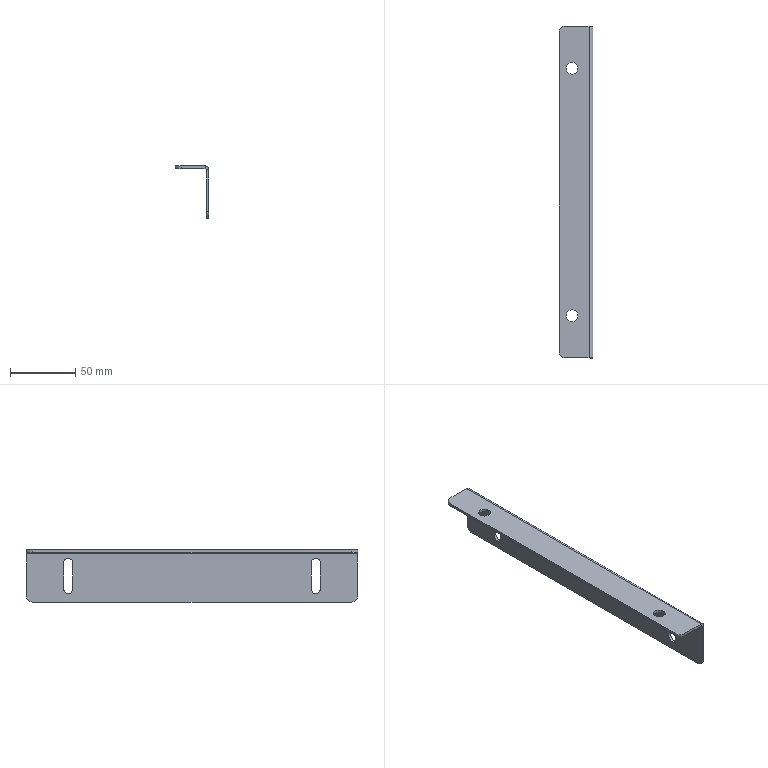Part | SolidWorks | features ICE 2, EdgeFlange 1, Fillet 1, FlatPattern 1, SMBaseFlange 1, SheetMetal 1 | 1 solid | 32 faces | box 26 x 255 x 40 mm | volume 31191 mm3 | cylinder 16 | plane 16 | commonest cylinder face diameters 7 x6 9 x4 10 x4 2 x1 6 x1
STEP:
#1=CARTESIAN_POINT('',(-7.5,95.,-2.));
#2=VERTEX_POINT('',#1);
#3=CARTESIAN_POINT('',(1.5,95.,-2.));
#4=VERTEX_POINT('',#3);
#5=CARTESIAN_POINT('',(-3.,95.,-2.));
#6=DIRECTION('',(0.,0.,1.));
#7=DIRECTION('',(1.,0.,0.));
#8=AXIS2_PLACEMENT_3D('',#5,#6,#7);
#9=CIRCLE('',#8,4.5);
#10=EDGE_CURVE('',#2,#4,#9,.T.);
#11=ORIENTED_EDGE('',*,*,#10,.F.);
#12=CARTESIAN_POINT('',(-7.5,95.,0.));
#13=VERTEX_POINT('',#12);
#14=CARTESIAN_POINT('',(-7.5,95.,-10.));
#15=DIRECTION('',(0.,0.,1.));
#16=VECTOR('',#15,1000.);
#17=LINE('',#14,#16);
#18=EDGE_CURVE('',#2,#13,#17,.T.);
#19=ORIENTED_EDGE('',*,*,#18,.T.);
#20=CARTESIAN_POINT('',(1.5,95.,0.));
#21=VERTEX_POINT('',#20);
#22=CARTESIAN_POINT('',(-3.,95.,0.));
#23=DIRECTION('',(0.,0.,1.));
#24=DIRECTION('',(1.,0.,0.));
#25=AXIS2_PLACEMENT_3D('',#22,#23,#24);
#26=CIRCLE('',#25,4.5);
#27=EDGE_CURVE('',#13,#21,#26,.T.);
#28=ORIENTED_EDGE('',*,*,#27,.T.);
#29=CARTESIAN_POINT('',(1.5,95.,-10.));
#30=DIRECTION('',(0.,0.,1.));
#31=VECTOR('',#30,1000.);
#32=LINE('',#29,#31);
#33=EDGE_CURVE('',#4,#21,#32,.T.);
#34=ORIENTED_EDGE('',*,*,#33,.F.);
#35=EDGE_LOOP('',(#11,#19,#28,#34));
#36=FACE_OUTER_BOUND('',#35,.T.);
#37=CARTESIAN_POINT('',(-3.,95.,-10.));
#38=DIRECTION('',(0.,0.,1.));
#39=DIRECTION('',(1.,0.,0.));
#40=AXIS2_PLACEMENT_3D('',#37,#38,#39);
#41=CYLINDRICAL_SURFACE('',#40,4.5);
#42=ADVANCED_FACE('',(#36),#41,.F.);
#43=CARTESIAN_POINT('',(-7.5,-95.,-2.));
#44=VERTEX_POINT('',#43);
#45=CARTESIAN_POINT('',(1.5,-95.,-2.));
#46=VERTEX_POINT('',#45);
#47=CARTESIAN_POINT('',(-3.,-95.,-2.));
#48=DIRECTION('',(0.,0.,1.));
#49=DIRECTION('',(1.,0.,0.));
#50=AXIS2_PLACEMENT_3D('',#47,#48,#49);
#51=CIRCLE('',#50,4.5);
#52=EDGE_CURVE('',#44,#46,#51,.T.);
#53=ORIENTED_EDGE('',*,*,#52,.F.);
#54=CARTESIAN_POINT('',(-7.5,-95.,0.));
#55=VERTEX_POINT('',#54);
#56=CARTESIAN_POINT('',(-7.5,-95.,-10.));
#57=DIRECTION('',(0.,0.,1.));
#58=VECTOR('',#57,1000.);
#59=LINE('',#56,#58);
#60=EDGE_CURVE('',#44,#55,#59,.T.);
#61=ORIENTED_EDGE('',*,*,#60,.T.);
#62=CARTESIAN_POINT('',(1.5,-95.,0.));
#63=VERTEX_POINT('',#62);
#64=CARTESIAN_POINT('',(-3.,-95.,0.));
#65=DIRECTION('',(0.,0.,1.));
#66=DIRECTION('',(-1.,0.,0.));
#67=AXIS2_PLACEMENT_3D('',#64,#65,#66);
#68=CIRCLE('',#67,4.5);
#69=EDGE_CURVE('',#55,#63,#68,.T.);
#70=ORIENTED_EDGE('',*,*,#69,.T.);
#71=CARTESIAN_POINT('',(1.5,-95.,-10.));
#72=DIRECTION('',(0.,0.,1.));
#73=VECTOR('',#72,1000.);
#74=LINE('',#71,#73);
#75=EDGE_CURVE('',#46,#63,#74,.T.);
#76=ORIENTED_EDGE('',*,*,#75,.F.);
#77=EDGE_LOOP('',(#53,#61,#70,#76));
#78=FACE_OUTER_BOUND('',#77,.T.);
#79=CARTESIAN_POINT('',(-3.,-95.,-10.));
#80=DIRECTION('',(0.,0.,1.));
#81=DIRECTION('',(1.,0.,0.));
#82=AXIS2_PLACEMENT_3D('',#79,#80,#81);
#83=CYLINDRICAL_SURFACE('',#82,4.5);
#84=ADVANCED_FACE('',(#78),#83,.F.);
#85=CARTESIAN_POINT('',(11.,95.,-33.5));
#86=VERTEX_POINT('',#85);
#87=CARTESIAN_POINT('',(11.,98.5,-30.));
#88=VERTEX_POINT('',#87);
#89=CARTESIAN_POINT('',(11.,95.,-30.));
#90=DIRECTION('',(1.,0.,0.));
#91=DIRECTION('',(0.,0.,-1.));
#92=AXIS2_PLACEMENT_3D('',#89,#90,#91);
#93=CIRCLE('',#92,3.5);
#94=EDGE_CURVE('',#86,#88,#93,.T.);
#95=ORIENTED_EDGE('',*,*,#94,.F.);
#96=CARTESIAN_POINT('',(13.,95.,-33.5));
#97=VERTEX_POINT('',#96);
#98=CARTESIAN_POINT('',(3.,95.,-33.5));
#99=DIRECTION('',(1.,0.,0.));
#100=VECTOR('',#99,1000.);
#101=LINE('',#98,#100);
#102=EDGE_CURVE('',#86,#97,#101,.T.);
#103=ORIENTED_EDGE('',*,*,#102,.T.);
#104=CARTESIAN_POINT('',(13.,98.5,-30.));
#105=VERTEX_POINT('',#104);
#106=CARTESIAN_POINT('',(13.,95.,-30.));
#107=DIRECTION('',(1.,0.,0.));
#108=DIRECTION('',(0.,0.,-1.));
#109=AXIS2_PLACEMENT_3D('',#106,#107,#108);
#110=CIRCLE('',#109,3.5);
#111=EDGE_CURVE('',#97,#105,#110,.T.);
#112=ORIENTED_EDGE('',*,*,#111,.T.);
#113=CARTESIAN_POINT('',(3.,98.5,-30.));
#114=DIRECTION('',(1.,0.,0.));
#115=VECTOR('',#114,1000.);
#116=LINE('',#113,#115);
#117=EDGE_CURVE('',#88,#105,#116,.T.);
#118=ORIENTED_EDGE('',*,*,#117,.F.);
#119=EDGE_LOOP('',(#95,#103,#112,#118));
#120=FACE_OUTER_BOUND('',#119,.T.);
#121=CARTESIAN_POINT('',(3.,95.,-30.));
#122=DIRECTION('',(1.,0.,0.));
#123=DIRECTION('',(0.,0.,-1.));
#124=AXIS2_PLACEMENT_3D('',#121,#122,#123);
#125=CYLINDRICAL_SURFACE('',#124,3.5);
#126=ADVANCED_FACE('',(#120),#125,.F.);
#127=CARTESIAN_POINT('',(11.,-95.,-33.5));
#128=VERTEX_POINT('',#127);
#129=CARTESIAN_POINT('',(11.,-91.5,-30.));
#130=VERTEX_POINT('',#129);
#131=CARTESIAN_POINT('',(11.,-95.,-30.));
#132=DIRECTION('',(1.,0.,0.));
#133=DIRECTION('',(0.,0.,-1.));
#134=AXIS2_PLACEMENT_3D('',#131,#132,#133);
#135=CIRCLE('',#134,3.5);
#136=EDGE_CURVE('',#128,#130,#135,.T.);
#137=ORIENTED_EDGE('',*,*,#136,.F.);
#138=CARTESIAN_POINT('',(13.,-95.,-33.5));
#139=VERTEX_POINT('',#138);
#140=CARTESIAN_POINT('',(3.,-95.,-33.5));
#141=DIRECTION('',(1.,0.,0.));
#142=VECTOR('',#141,1000.);
#143=LINE('',#140,#142);
#144=EDGE_CURVE('',#128,#139,#143,.T.);
#145=ORIENTED_EDGE('',*,*,#144,.T.);
#146=CARTESIAN_POINT('',(13.,-91.5,-30.));
#147=VERTEX_POINT('',#146);
#148=CARTESIAN_POINT('',(13.,-95.,-30.));
#149=DIRECTION('',(1.,0.,0.));
#150=DIRECTION('',(0.,0.,1.));
#151=AXIS2_PLACEMENT_3D('',#148,#149,#150);
#152=CIRCLE('',#151,3.5);
#153=EDGE_CURVE('',#139,#147,#152,.T.);
#154=ORIENTED_EDGE('',*,*,#153,.T.);
#155=CARTESIAN_POINT('',(3.,-91.5,-30.));
#156=DIRECTION('',(1.,0.,0.));
#157=VECTOR('',#156,1000.);
#158=LINE('',#155,#157);
#159=EDGE_CURVE('',#130,#147,#158,.T.);
#160=ORIENTED_EDGE('',*,*,#159,.F.);
#161=EDGE_LOOP('',(#137,#145,#154,#160));
#162=FACE_OUTER_BOUND('',#161,.T.);
#163=CARTESIAN_POINT('',(3.,-95.,-30.));
#164=DIRECTION('',(1.,0.,0.));
#165=DIRECTION('',(0.,0.,-1.));
#166=AXIS2_PLACEMENT_3D('',#163,#164,#165);
#167=CYLINDRICAL_SURFACE('',#166,3.5);
#168=ADVANCED_FACE('',(#162),#167,.F.);
#169=CARTESIAN_POINT('',(-8.,-127.5,0.));
#170=VERTEX_POINT('',#169);
#171=CARTESIAN_POINT('',(10.,-127.5,0.));
#172=VERTEX_POINT('',#171);
#173=CARTESIAN_POINT('',(-13.,-127.5,0.));
#174=DIRECTION('',(1.,0.,0.));
#175=VECTOR('',#174,1000.);
#176=LINE('',#173,#175);
#177=EDGE_CURVE('',#170,#172,#176,.T.);
#178=ORIENTED_EDGE('',*,*,#177,.F.);
#179=CARTESIAN_POINT('',(-8.,-127.5,-2.));
#180=VERTEX_POINT('',#179);
#181=CARTESIAN_POINT('',(-8.,-127.5,-2.));
#182=DIRECTION('',(0.,0.,-1.));
#183=VECTOR('',#182,1000.);
#184=LINE('',#181,#183);
#185=EDGE_CURVE('',#170,#180,#184,.T.);
#186=ORIENTED_EDGE('',*,*,#185,.T.);
#187=CARTESIAN_POINT('',(10.,-127.5,-2.));
#188=VERTEX_POINT('',#187);
#189=CARTESIAN_POINT('',(-13.,-127.5,-2.));
#190=DIRECTION('',(1.,0.,0.));
#191=VECTOR('',#190,1000.);
#192=LINE('',#189,#191);
#193=EDGE_CURVE('',#180,#188,#192,.T.);
#194=ORIENTED_EDGE('',*,*,#193,.T.);
#195=CARTESIAN_POINT('',(10.,-127.5,-2.));
#196=DIRECTION('',(0.,0.,1.));
#197=VECTOR('',#196,1000.);
#198=LINE('',#195,#197);
#199=EDGE_CURVE('',#188,#172,#198,.T.);
#200=ORIENTED_EDGE('',*,*,#199,.T.);
#201=EDGE_LOOP('',(#178,#186,#194,#200));
#202=FACE_OUTER_BOUND('',#201,.T.);
#203=CARTESIAN_POINT('',(-13.,-127.5,-2.));
#204=DIRECTION('',(0.,-1.,0.));
#205=DIRECTION('',(0.,0.,-1.));
#206=AXIS2_PLACEMENT_3D('',#203,#204,#205);
#207=PLANE('',#206);
#208=ADVANCED_FACE('',(#202),#207,.T.);
#209=CARTESIAN_POINT('',(-3.,95.,-2.));
#210=DIRECTION('',(0.,0.,1.));
#211=DIRECTION('',(1.,0.,0.));
#212=AXIS2_PLACEMENT_3D('',#209,#210,#211);
#213=CIRCLE('',#212,4.5);
#214=EDGE_CURVE('',#4,#2,#213,.T.);
#215=ORIENTED_EDGE('',*,*,#214,.T.);
#216=ORIENTED_EDGE('',*,*,#10,.T.);
#217=EDGE_LOOP('',(#215,#216));
#218=FACE_BOUND('',#217,.T.);
#219=CARTESIAN_POINT('',(-3.,-95.,-2.));
#220=DIRECTION('',(0.,0.,1.));
#221=DIRECTION('',(1.,0.,0.));
#222=AXIS2_PLACEMENT_3D('',#219,#220,#221);
#223=CIRCLE('',#222,4.5);
#224=EDGE_CURVE('',#46,#44,#223,.T.);
#225=ORIENTED_EDGE('',*,*,#224,.T.);
#226=ORIENTED_EDGE('',*,*,#52,.T.);
#227=EDGE_LOOP('',(#225,#226));
#228=FACE_BOUND('',#227,.T.);
#229=ORIENTED_EDGE('',*,*,#193,.F.);
#230=CARTESIAN_POINT('',(-13.,-122.5,-2.));
#231=VERTEX_POINT('',#230);
#232=CARTESIAN_POINT('',(-8.,-122.5,-2.));
#233=DIRECTION('',(0.,0.,-1.));
#234=DIRECTION('',(1.,0.,0.));
#235=AXIS2_PLACEMENT_3D('',#232,#233,#234);
#236=CIRCLE('',#235,5.);
#237=EDGE_CURVE('',#180,#231,#236,.T.);
#238=ORIENTED_EDGE('',*,*,#237,.T.);
#239=CARTESIAN_POINT('',(-13.,122.5,-2.));
#240=VERTEX_POINT('',#239);
#241=CARTESIAN_POINT('',(-13.,127.5,-2.));
#242=DIRECTION('',(0.,-1.,0.));
#243=VECTOR('',#242,1000.);
#244=LINE('',#241,#243);
#245=EDGE_CURVE('',#240,#231,#244,.T.);
#246=ORIENTED_EDGE('',*,*,#245,.F.);
#247=CARTESIAN_POINT('',(-8.,127.5,-2.));
#248=VERTEX_POINT('',#247);
#249=CARTESIAN_POINT('',(-8.,122.5,-2.));
#250=DIRECTION('',(0.,0.,-1.));
#251=DIRECTION('',(1.,0.,0.));
#252=AXIS2_PLACEMENT_3D('',#249,#250,#251);
#253=CIRCLE('',#252,5.);
#254=EDGE_CURVE('',#240,#248,#253,.T.);
#255=ORIENTED_EDGE('',*,*,#254,.T.);
#256=CARTESIAN_POINT('',(10.,127.5,-2.));
#257=VERTEX_POINT('',#256);
#258=CARTESIAN_POINT('',(-13.,127.5,-2.));
#259=DIRECTION('',(-1.,0.,0.));
#260=VECTOR('',#259,1000.);
#261=LINE('',#258,#260);
#262=EDGE_CURVE('',#257,#248,#261,.T.);
#263=ORIENTED_EDGE('',*,*,#262,.F.);
#264=CARTESIAN_POINT('',(10.,-127.5,-2.));
#265=DIRECTION('',(0.,1.,0.));
#266=VECTOR('',#265,1000.);
#267=LINE('',#264,#266);
#268=EDGE_CURVE('',#188,#257,#267,.T.);
#269=ORIENTED_EDGE('',*,*,#268,.F.);
#270=EDGE_LOOP('',(#229,#238,#246,#255,#263,#269));
#271=FACE_OUTER_BOUND('',#270,.T.);
#272=CARTESIAN_POINT('',(0.,0.,-2.));
#273=DIRECTION('',(0.,0.,1.));
#274=DIRECTION('',(1.,0.,0.));
#275=AXIS2_PLACEMENT_3D('',#272,#273,#274);
#276=PLANE('',#275);
#277=ADVANCED_FACE('',(#218,#228,#271),#276,.F.);
#278=CARTESIAN_POINT('',(-3.,95.,0.));
#279=DIRECTION('',(0.,0.,1.));
#280=DIRECTION('',(1.,0.,0.));
#281=AXIS2_PLACEMENT_3D('',#278,#279,#280);
#282=CIRCLE('',#281,4.5);
#283=EDGE_CURVE('',#21,#13,#282,.T.);
#284=ORIENTED_EDGE('',*,*,#283,.F.);
#285=ORIENTED_EDGE('',*,*,#27,.F.);
#286=EDGE_LOOP('',(#284,#285));
#287=FACE_BOUND('',#286,.T.);
#288=CARTESIAN_POINT('',(-3.,-95.,0.));
#289=DIRECTION('',(0.,0.,1.));
#290=DIRECTION('',(-1.,0.,0.));
#291=AXIS2_PLACEMENT_3D('',#288,#289,#290);
#292=CIRCLE('',#291,4.5);
#293=EDGE_CURVE('',#63,#55,#292,.T.);
#294=ORIENTED_EDGE('',*,*,#293,.F.);
#295=ORIENTED_EDGE('',*,*,#69,.F.);
#296=EDGE_LOOP('',(#294,#295));
#297=FACE_BOUND('',#296,.T.);
#298=CARTESIAN_POINT('',(-13.,122.5,0.));
#299=VERTEX_POINT('',#298);
#300=CARTESIAN_POINT('',(-13.,-122.5,0.));
#301=VERTEX_POINT('',#300);
#302=CARTESIAN_POINT('',(-13.,127.5,0.));
#303=DIRECTION('',(0.,-1.,0.));
#304=VECTOR('',#303,1000.);
#305=LINE('',#302,#304);
#306=EDGE_CURVE('',#299,#301,#305,.T.);
#307=ORIENTED_EDGE('',*,*,#306,.T.);
#308=CARTESIAN_POINT('',(-8.,-122.5,0.));
#309=DIRECTION('',(0.,0.,1.));
#310=DIRECTION('',(1.,0.,0.));
#311=AXIS2_PLACEMENT_3D('',#308,#309,#310);
#312=CIRCLE('',#311,5.);
#313=EDGE_CURVE('',#301,#170,#312,.T.);
#314=ORIENTED_EDGE('',*,*,#313,.T.);
#315=ORIENTED_EDGE('',*,*,#177,.T.);
#316=CARTESIAN_POINT('',(10.,127.5,0.));
#317=VERTEX_POINT('',#316);
#318=CARTESIAN_POINT('',(10.,-127.5,0.));
#319=DIRECTION('',(0.,1.,0.));
#320=VECTOR('',#319,1000.);
#321=LINE('',#318,#320);
#322=EDGE_CURVE('',#172,#317,#321,.T.);
#323=ORIENTED_EDGE('',*,*,#322,.T.);
#324=CARTESIAN_POINT('',(-8.,127.5,0.));
#325=VERTEX_POINT('',#324);
#326=CARTESIAN_POINT('',(-13.,127.5,0.));
#327=DIRECTION('',(-1.,0.,0.));
#328=VECTOR('',#327,1000.);
#329=LINE('',#326,#328);
#330=EDGE_CURVE('',#317,#325,#329,.T.);
#331=ORIENTED_EDGE('',*,*,#330,.T.);
#332=CARTESIAN_POINT('',(-8.,122.5,0.));
#333=DIRECTION('',(0.,0.,1.));
#334=DIRECTION('',(1.,0.,0.));
#335=AXIS2_PLACEMENT_3D('',#332,#333,#334);
#336=CIRCLE('',#335,5.);
#337=EDGE_CURVE('',#325,#299,#336,.T.);
#338=ORIENTED_EDGE('',*,*,#337,.T.);
#339=EDGE_LOOP('',(#307,#314,#315,#323,#331,#338));
#340=FACE_OUTER_BOUND('',#339,.T.);
#341=CARTESIAN_POINT('',(0.,0.,0.));
#342=DIRECTION('',(0.,0.,1.));
#343=DIRECTION('',(1.,0.,0.));
#344=AXIS2_PLACEMENT_3D('',#341,#342,#343);
#345=PLANE('',#344);
#346=ADVANCED_FACE('',(#287,#297,#340),#345,.T.);
#347=ORIENTED_EDGE('',*,*,#245,.T.);
#348=CARTESIAN_POINT('',(-13.,-122.5,-2.));
#349=DIRECTION('',(0.,0.,1.));
#350=VECTOR('',#349,1000.);
#351=LINE('',#348,#350);
#352=EDGE_CURVE('',#231,#301,#351,.T.);
#353=ORIENTED_EDGE('',*,*,#352,.T.);
#354=ORIENTED_EDGE('',*,*,#306,.F.);
#355=CARTESIAN_POINT('',(-13.,122.5,-2.));
#356=DIRECTION('',(0.,0.,-1.));
#357=VECTOR('',#356,1000.);
#358=LINE('',#355,#357);
#359=EDGE_CURVE('',#299,#240,#358,.T.);
#360=ORIENTED_EDGE('',*,*,#359,.T.);
#361=EDGE_LOOP('',(#347,#353,#354,#360));
#362=FACE_OUTER_BOUND('',#361,.T.);
#363=CARTESIAN_POINT('',(-13.,127.5,-2.));
#364=DIRECTION('',(-1.,0.,0.));
#365=DIRECTION('',(0.,-1.,0.));
#366=AXIS2_PLACEMENT_3D('',#363,#364,#365);
#367=PLANE('',#366);
#368=ADVANCED_FACE('',(#362),#367,.T.);
#369=ORIENTED_EDGE('',*,*,#262,.T.);
#370=CARTESIAN_POINT('',(-8.,127.5,-2.));
#371=DIRECTION('',(0.,0.,1.));
#372=VECTOR('',#371,1000.);
#373=LINE('',#370,#372);
#374=EDGE_CURVE('',#248,#325,#373,.T.);
#375=ORIENTED_EDGE('',*,*,#374,.T.);
#376=ORIENTED_EDGE('',*,*,#330,.F.);
#377=CARTESIAN_POINT('',(10.,127.5,-2.));
#378=DIRECTION('',(0.,0.,1.));
#379=VECTOR('',#378,1000.);
#380=LINE('',#377,#379);
#381=EDGE_CURVE('',#257,#317,#380,.T.);
#382=ORIENTED_EDGE('',*,*,#381,.F.);
#383=EDGE_LOOP('',(#369,#375,#376,#382));
#384=FACE_OUTER_BOUND('',#383,.T.);
#385=CARTESIAN_POINT('',(-13.,127.5,-2.));
#386=DIRECTION('',(0.,1.,0.));
#387=DIRECTION('',(0.,0.,1.));
#388=AXIS2_PLACEMENT_3D('',#385,#386,#387);
#389=PLANE('',#388);
#390=ADVANCED_FACE('',(#384),#389,.T.);
#391=CARTESIAN_POINT('',(11.,127.5,-3.));
#392=VERTEX_POINT('',#391);
#393=CARTESIAN_POINT('',(13.,127.5,-3.));
#394=VERTEX_POINT('',#393);
#395=CARTESIAN_POINT('',(13.,127.5,-3.));
#396=DIRECTION('',(1.,0.,0.));
#397=VECTOR('',#396,1000.);
#398=LINE('',#395,#397);
#399=EDGE_CURVE('',#392,#394,#398,.T.);
#400=ORIENTED_EDGE('',*,*,#399,.F.);
#401=CARTESIAN_POINT('',(10.,127.5,-3.));
#402=DIRECTION('',(0.,1.,0.));
#403=DIRECTION('',(0.,0.,-1.));
#404=AXIS2_PLACEMENT_3D('',#401,#402,#403);
#405=CIRCLE('',#404,1.);
#406=EDGE_CURVE('',#257,#392,#405,.T.);
#407=ORIENTED_EDGE('',*,*,#406,.F.);
#408=ORIENTED_EDGE('',*,*,#381,.T.);
#409=CARTESIAN_POINT('',(10.,127.5,-3.));
#410=DIRECTION('',(0.,1.,0.));
#411=DIRECTION('',(0.,0.,-1.));
#412=AXIS2_PLACEMENT_3D('',#409,#410,#411);
#413=CIRCLE('',#412,3.);
#414=EDGE_CURVE('',#317,#394,#413,.T.);
#415=ORIENTED_EDGE('',*,*,#414,.T.);
#416=EDGE_LOOP('',(#400,#407,#408,#415));
#417=FACE_OUTER_BOUND('',#416,.T.);
#418=CARTESIAN_POINT('',(10.,127.5,-3.));
#419=DIRECTION('',(0.,1.,0.));
#420=DIRECTION('',(0.,0.,1.));
#421=AXIS2_PLACEMENT_3D('',#418,#419,#420);
#422=PLANE('',#421);
#423=ADVANCED_FACE('',(#417),#422,.T.);
#424=CARTESIAN_POINT('',(11.,-127.5,-3.));
#425=VERTEX_POINT('',#424);
#426=CARTESIAN_POINT('',(10.,-127.5,-3.));
#427=DIRECTION('',(0.,-1.,0.));
#428=DIRECTION('',(0.,0.,-1.));
#429=AXIS2_PLACEMENT_3D('',#426,#427,#428);
#430=CIRCLE('',#429,1.);
#431=EDGE_CURVE('',#425,#188,#430,.T.);
#432=ORIENTED_EDGE('',*,*,#431,.F.);
#433=CARTESIAN_POINT('',(13.,-127.5,-3.));
#434=VERTEX_POINT('',#433);
#435=CARTESIAN_POINT('',(11.,-127.5,-3.));
#436=DIRECTION('',(1.,0.,0.));
#437=VECTOR('',#436,1000.);
#438=LINE('',#435,#437);
#439=EDGE_CURVE('',#425,#434,#438,.T.);
#440=ORIENTED_EDGE('',*,*,#439,.T.);
#441=CARTESIAN_POINT('',(10.,-127.5,-3.));
#442=DIRECTION('',(0.,-1.,0.));
#443=DIRECTION('',(0.,0.,-1.));
#444=AXIS2_PLACEMENT_3D('',#441,#442,#443);
#445=CIRCLE('',#444,3.);
#446=EDGE_CURVE('',#434,#172,#445,.T.);
#447=ORIENTED_EDGE('',*,*,#446,.T.);
#448=ORIENTED_EDGE('',*,*,#199,.F.);
#449=EDGE_LOOP('',(#432,#440,#447,#448));
#450=FACE_OUTER_BOUND('',#449,.T.);
#451=CARTESIAN_POINT('',(10.,-127.5,-3.));
#452=DIRECTION('',(0.,1.,0.));
#453=DIRECTION('',(0.,0.,1.));
#454=AXIS2_PLACEMENT_3D('',#451,#452,#453);
#455=PLANE('',#454);
#456=ADVANCED_FACE('',(#450),#455,.F.);
#457=ORIENTED_EDGE('',*,*,#322,.F.);
#458=ORIENTED_EDGE('',*,*,#446,.F.);
#459=CARTESIAN_POINT('',(13.,0.,-3.));
#460=DIRECTION('',(0.,-1.,0.));
#461=VECTOR('',#460,1000.);
#462=LINE('',#459,#461);
#463=EDGE_CURVE('',#394,#434,#462,.T.);
#464=ORIENTED_EDGE('',*,*,#463,.F.);
#465=ORIENTED_EDGE('',*,*,#414,.F.);
#466=EDGE_LOOP('',(#457,#458,#464,#465));
#467=FACE_OUTER_BOUND('',#466,.T.);
#468=CARTESIAN_POINT('',(10.,-127.5,-3.));
#469=DIRECTION('',(0.,-1.,0.));
#470=DIRECTION('',(1.,0.,0.));
#471=AXIS2_PLACEMENT_3D('',#468,#469,#470);
#472=CYLINDRICAL_SURFACE('',#471,3.);
#473=ADVANCED_FACE('',(#467),#472,.T.);
#474=ORIENTED_EDGE('',*,*,#268,.T.);
#475=ORIENTED_EDGE('',*,*,#406,.T.);
#476=CARTESIAN_POINT('',(11.,127.5,-3.));
#477=DIRECTION('',(0.,-1.,0.));
#478=VECTOR('',#477,1000.);
#479=LINE('',#476,#478);
#480=EDGE_CURVE('',#392,#425,#479,.T.);
#481=ORIENTED_EDGE('',*,*,#480,.T.);
#482=ORIENTED_EDGE('',*,*,#431,.T.);
#483=EDGE_LOOP('',(#474,#475,#481,#482));
#484=FACE_OUTER_BOUND('',#483,.T.);
#485=CARTESIAN_POINT('',(10.,-127.5,-3.));
#486=DIRECTION('',(0.,-1.,0.));
#487=DIRECTION('',(1.,0.,0.));
#488=AXIS2_PLACEMENT_3D('',#485,#486,#487);
#489=CYLINDRICAL_SURFACE('',#488,1.);
#490=ADVANCED_FACE('',(#484),#489,.F.);
#491=CARTESIAN_POINT('',(11.,-127.5,-35.));
#492=VERTEX_POINT('',#491);
#493=CARTESIAN_POINT('',(11.,-127.5,0.));
#494=DIRECTION('',(0.,0.,1.));
#495=VECTOR('',#494,1000.);
#496=LINE('',#493,#495);
#497=EDGE_CURVE('',#492,#425,#496,.T.);
#498=ORIENTED_EDGE('',*,*,#497,.F.);
#499=CARTESIAN_POINT('',(13.,-127.5,-35.));
#500=VERTEX_POINT('',#499);
#501=CARTESIAN_POINT('',(13.,-127.5,-35.));
#502=DIRECTION('',(1.,0.,0.));
#503=VECTOR('',#502,1000.);
#504=LINE('',#501,#503);
#505=EDGE_CURVE('',#492,#500,#504,.T.);
#506=ORIENTED_EDGE('',*,*,#505,.T.);
#507=CARTESIAN_POINT('',(13.,-127.5,-2.));
#508=DIRECTION('',(0.,0.,1.));
#509=VECTOR('',#508,1000.);
#510=LINE('',#507,#509);
#511=EDGE_CURVE('',#500,#434,#510,.T.);
#512=ORIENTED_EDGE('',*,*,#511,.T.);
#513=ORIENTED_EDGE('',*,*,#439,.F.);
#514=EDGE_LOOP('',(#498,#506,#512,#513));
#515=FACE_OUTER_BOUND('',#514,.T.);
#516=CARTESIAN_POINT('',(13.,-127.5,-2.));
#517=DIRECTION('',(0.,-1.,0.));
#518=DIRECTION('',(1.,0.,0.));
#519=AXIS2_PLACEMENT_3D('',#516,#517,#518);
#520=PLANE('',#519);
#521=ADVANCED_FACE('',(#515),#520,.T.);
#522=CARTESIAN_POINT('',(13.,127.5,-35.));
#523=VERTEX_POINT('',#522);
#524=CARTESIAN_POINT('',(13.,127.5,-40.));
#525=DIRECTION('',(0.,0.,-1.));
#526=VECTOR('',#525,1000.);
#527=LINE('',#524,#526);
#528=EDGE_CURVE('',#394,#523,#527,.T.);
#529=ORIENTED_EDGE('',*,*,#528,.T.);
#530=CARTESIAN_POINT('',(11.,127.5,-35.));
#531=VERTEX_POINT('',#530);
#532=CARTESIAN_POINT('',(13.,127.5,-35.));
#533=DIRECTION('',(-1.,0.,0.));
#534=VECTOR('',#533,1000.);
#535=LINE('',#532,#534);
#536=EDGE_CURVE('',#523,#531,#535,.T.);
#537=ORIENTED_EDGE('',*,*,#536,.T.);
#538=CARTESIAN_POINT('',(11.,127.5,0.));
#539=DIRECTION('',(0.,0.,-1.));
#540=VECTOR('',#539,1000.);
#541=LINE('',#538,#540);
#542=EDGE_CURVE('',#392,#531,#541,.T.);
#543=ORIENTED_EDGE('',*,*,#542,.F.);
#544=ORIENTED_EDGE('',*,*,#399,.T.);
#545=EDGE_LOOP('',(#529,#537,#543,#544));
#546=FACE_OUTER_BOUND('',#545,.T.);
#547=CARTESIAN_POINT('',(13.,127.5,-40.));
#548=DIRECTION('',(0.,1.,0.));
#549=DIRECTION('',(-1.,0.,0.));
#550=AXIS2_PLACEMENT_3D('',#547,#548,#549);
#551=PLANE('',#550);
#552=ADVANCED_FACE('',(#546),#551,.T.);
#553=CARTESIAN_POINT('',(13.,98.5,-10.));
#554=VERTEX_POINT('',#553);
#555=CARTESIAN_POINT('',(13.,91.5,-10.));
#556=VERTEX_POINT('',#555);
#557=CARTESIAN_POINT('',(13.,95.,-10.));
#558=DIRECTION('',(1.,0.,0.));
#559=DIRECTION('',(0.,0.,-1.));
#560=AXIS2_PLACEMENT_3D('',#557,#558,#559);
#561=CIRCLE('',#560,3.5);
#562=EDGE_CURVE('',#554,#556,#561,.T.);
#563=ORIENTED_EDGE('',*,*,#562,.F.);
#564=CARTESIAN_POINT('',(13.,98.5,-10.));
#565=DIRECTION('',(0.,0.,1.));
#566=VECTOR('',#565,1000.);
#567=LINE('',#564,#566);
#568=EDGE_CURVE('',#105,#554,#567,.T.);
#569=ORIENTED_EDGE('',*,*,#568,.F.);
#570=ORIENTED_EDGE('',*,*,#111,.F.);
#571=CARTESIAN_POINT('',(13.,91.5,-30.));
#572=VERTEX_POINT('',#571);
#573=CARTESIAN_POINT('',(13.,95.,-30.));
#574=DIRECTION('',(1.,0.,0.));
#575=DIRECTION('',(0.,0.,-1.));
#576=AXIS2_PLACEMENT_3D('',#573,#574,#575);
#577=CIRCLE('',#576,3.5);
#578=EDGE_CURVE('',#572,#97,#577,.T.);
#579=ORIENTED_EDGE('',*,*,#578,.F.);
#580=CARTESIAN_POINT('',(13.,91.5,-10.));
#581=DIRECTION('',(0.,0.,-1.));
#582=VECTOR('',#581,1000.);
#583=LINE('',#580,#582);
#584=EDGE_CURVE('',#556,#572,#583,.T.);
#585=ORIENTED_EDGE('',*,*,#584,.F.);
#586=EDGE_LOOP('',(#563,#569,#570,#579,#585));
#587=FACE_BOUND('',#586,.T.);
#588=CARTESIAN_POINT('',(13.,-91.5,-10.));
#589=VERTEX_POINT('',#588);
#590=CARTESIAN_POINT('',(13.,-98.5,-10.));
#591=VERTEX_POINT('',#590);
#592=CARTESIAN_POINT('',(13.,-95.,-10.));
#593=DIRECTION('',(1.,0.,0.));
#594=DIRECTION('',(0.,0.,1.));
#595=AXIS2_PLACEMENT_3D('',#592,#593,#594);
#596=CIRCLE('',#595,3.5);
#597=EDGE_CURVE('',#589,#591,#596,.T.);
#598=ORIENTED_EDGE('',*,*,#597,.F.);
#599=CARTESIAN_POINT('',(13.,-91.5,-10.));
#600=DIRECTION('',(0.,0.,1.));
#601=VECTOR('',#600,1000.);
#602=LINE('',#599,#601);
#603=EDGE_CURVE('',#147,#589,#602,.T.);
#604=ORIENTED_EDGE('',*,*,#603,.F.);
#605=ORIENTED_EDGE('',*,*,#153,.F.);
#606=CARTESIAN_POINT('',(13.,-98.5,-30.));
#607=VERTEX_POINT('',#606);
#608=CARTESIAN_POINT('',(13.,-95.,-30.));
#609=DIRECTION('',(1.,0.,0.));
#610=DIRECTION('',(0.,0.,1.));
#611=AXIS2_PLACEMENT_3D('',#608,#609,#610);
#612=CIRCLE('',#611,3.5);
#613=EDGE_CURVE('',#607,#139,#612,.T.);
#614=ORIENTED_EDGE('',*,*,#613,.F.);
#615=CARTESIAN_POINT('',(13.,-98.5,-10.));
#616=DIRECTION('',(0.,0.,-1.));
#617=VECTOR('',#616,1000.);
#618=LINE('',#615,#617);
#619=EDGE_CURVE('',#591,#607,#618,.T.);
#620=ORIENTED_EDGE('',*,*,#619,.F.);
#621=EDGE_LOOP('',(#598,#604,#605,#614,#620));
#622=FACE_BOUND('',#621,.T.);
#623=ORIENTED_EDGE('',*,*,#511,.F.);
#624=CARTESIAN_POINT('',(13.,-122.5,-40.));
#625=VERTEX_POINT('',#624);
#626=CARTESIAN_POINT('',(13.,-122.5,-35.));
#627=DIRECTION('',(1.,0.,0.));
#628=DIRECTION('',(0.,0.,-1.));
#629=AXIS2_PLACEMENT_3D('',#626,#627,#628);
#630=CIRCLE('',#629,5.);
#631=EDGE_CURVE('',#500,#625,#630,.T.);
#632=ORIENTED_EDGE('',*,*,#631,.T.);
#633=CARTESIAN_POINT('',(13.,122.5,-40.));
#634=VERTEX_POINT('',#633);
#635=CARTESIAN_POINT('',(13.,-127.5,-40.));
#636=DIRECTION('',(0.,-1.,0.));
#637=VECTOR('',#636,1000.);
#638=LINE('',#635,#637);
#639=EDGE_CURVE('',#634,#625,#638,.T.);
#640=ORIENTED_EDGE('',*,*,#639,.F.);
#641=CARTESIAN_POINT('',(13.,122.5,-35.));
#642=DIRECTION('',(1.,0.,0.));
#643=DIRECTION('',(0.,0.,-1.));
#644=AXIS2_PLACEMENT_3D('',#641,#642,#643);
#645=CIRCLE('',#644,5.);
#646=EDGE_CURVE('',#634,#523,#645,.T.);
#647=ORIENTED_EDGE('',*,*,#646,.T.);
#648=ORIENTED_EDGE('',*,*,#528,.F.);
#649=ORIENTED_EDGE('',*,*,#463,.T.);
#650=EDGE_LOOP('',(#623,#632,#640,#647,#648,#649));
#651=FACE_OUTER_BOUND('',#650,.T.);
#652=CARTESIAN_POINT('',(13.,0.,0.));
#653=DIRECTION('',(1.,0.,0.));
#654=DIRECTION('',(0.,0.,-1.));
#655=AXIS2_PLACEMENT_3D('',#652,#653,#654);
#656=PLANE('',#655);
#657=ADVANCED_FACE('',(#587,#622,#651),#656,.T.);
#658=CARTESIAN_POINT('',(11.,98.5,-10.));
#659=VERTEX_POINT('',#658);
#660=CARTESIAN_POINT('',(11.,98.5,0.));
#661=DIRECTION('',(0.,0.,1.));
#662=VECTOR('',#661,1000.);
#663=LINE('',#660,#662);
#664=EDGE_CURVE('',#88,#659,#663,.T.);
#665=ORIENTED_EDGE('',*,*,#664,.T.);
#666=CARTESIAN_POINT('',(11.,91.5,-10.));
#667=VERTEX_POINT('',#666);
#668=CARTESIAN_POINT('',(11.,95.,-10.));
#669=DIRECTION('',(1.,0.,0.));
#670=DIRECTION('',(0.,0.,-1.));
#671=AXIS2_PLACEMENT_3D('',#668,#669,#670);
#672=CIRCLE('',#671,3.5);
#673=EDGE_CURVE('',#659,#667,#672,.T.);
#674=ORIENTED_EDGE('',*,*,#673,.T.);
#675=CARTESIAN_POINT('',(11.,91.5,-30.));
#676=VERTEX_POINT('',#675);
#677=CARTESIAN_POINT('',(11.,91.5,0.));
#678=DIRECTION('',(0.,0.,-1.));
#679=VECTOR('',#678,1000.);
#680=LINE('',#677,#679);
#681=EDGE_CURVE('',#667,#676,#680,.T.);
#682=ORIENTED_EDGE('',*,*,#681,.T.);
#683=CARTESIAN_POINT('',(11.,95.,-30.));
#684=DIRECTION('',(1.,0.,0.));
#685=DIRECTION('',(0.,0.,-1.));
#686=AXIS2_PLACEMENT_3D('',#683,#684,#685);
#687=CIRCLE('',#686,3.5);
#688=EDGE_CURVE('',#676,#86,#687,.T.);
#689=ORIENTED_EDGE('',*,*,#688,.T.);
#690=ORIENTED_EDGE('',*,*,#94,.T.);
#691=EDGE_LOOP('',(#665,#674,#682,#689,#690));
#692=FACE_BOUND('',#691,.T.);
#693=CARTESIAN_POINT('',(11.,-91.5,-10.));
#694=VERTEX_POINT('',#693);
#695=CARTESIAN_POINT('',(11.,-91.5,0.));
#696=DIRECTION('',(0.,0.,1.));
#697=VECTOR('',#696,1000.);
#698=LINE('',#695,#697);
#699=EDGE_CURVE('',#130,#694,#698,.T.);
#700=ORIENTED_EDGE('',*,*,#699,.T.);
#701=CARTESIAN_POINT('',(11.,-98.5,-10.));
#702=VERTEX_POINT('',#701);
#703=CARTESIAN_POINT('',(11.,-95.,-10.));
#704=DIRECTION('',(1.,0.,0.));
#705=DIRECTION('',(0.,0.,-1.));
#706=AXIS2_PLACEMENT_3D('',#703,#704,#705);
#707=CIRCLE('',#706,3.5);
#708=EDGE_CURVE('',#694,#702,#707,.T.);
#709=ORIENTED_EDGE('',*,*,#708,.T.);
#710=CARTESIAN_POINT('',(11.,-98.5,-30.));
#711=VERTEX_POINT('',#710);
#712=CARTESIAN_POINT('',(11.,-98.5,0.));
#713=DIRECTION('',(0.,0.,-1.));
#714=VECTOR('',#713,1000.);
#715=LINE('',#712,#714);
#716=EDGE_CURVE('',#702,#711,#715,.T.);
#717=ORIENTED_EDGE('',*,*,#716,.T.);
#718=CARTESIAN_POINT('',(11.,-95.,-30.));
#719=DIRECTION('',(1.,0.,0.));
#720=DIRECTION('',(0.,0.,-1.));
#721=AXIS2_PLACEMENT_3D('',#718,#719,#720);
#722=CIRCLE('',#721,3.5);
#723=EDGE_CURVE('',#711,#128,#722,.T.);
#724=ORIENTED_EDGE('',*,*,#723,.T.);
#725=ORIENTED_EDGE('',*,*,#136,.T.);
#726=EDGE_LOOP('',(#700,#709,#717,#724,#725));
#727=FACE_BOUND('',#726,.T.);
#728=CARTESIAN_POINT('',(11.,122.5,-40.));
#729=VERTEX_POINT('',#728);
#730=CARTESIAN_POINT('',(11.,-122.5,-40.));
#731=VERTEX_POINT('',#730);
#732=CARTESIAN_POINT('',(11.,0.,-40.));
#733=DIRECTION('',(0.,-1.,0.));
#734=VECTOR('',#733,1000.);
#735=LINE('',#732,#734);
#736=EDGE_CURVE('',#729,#731,#735,.T.);
#737=ORIENTED_EDGE('',*,*,#736,.T.);
#738=CARTESIAN_POINT('',(11.,-122.5,-35.));
#739=DIRECTION('',(-1.,0.,0.));
#740=DIRECTION('',(0.,0.,-1.));
#741=AXIS2_PLACEMENT_3D('',#738,#739,#740);
#742=CIRCLE('',#741,5.);
#743=EDGE_CURVE('',#731,#492,#742,.T.);
#744=ORIENTED_EDGE('',*,*,#743,.T.);
#745=ORIENTED_EDGE('',*,*,#497,.T.);
#746=ORIENTED_EDGE('',*,*,#480,.F.);
#747=ORIENTED_EDGE('',*,*,#542,.T.);
#748=CARTESIAN_POINT('',(11.,122.5,-35.));
#749=DIRECTION('',(-1.,0.,0.));
#750=DIRECTION('',(0.,0.,-1.));
#751=AXIS2_PLACEMENT_3D('',#748,#749,#750);
#752=CIRCLE('',#751,5.);
#753=EDGE_CURVE('',#531,#729,#752,.T.);
#754=ORIENTED_EDGE('',*,*,#753,.T.);
#755=EDGE_LOOP('',(#737,#744,#745,#746,#747,#754));
#756=FACE_OUTER_BOUND('',#755,.T.);
#757=CARTESIAN_POINT('',(11.,0.,0.));
#758=DIRECTION('',(1.,0.,0.));
#759=DIRECTION('',(0.,0.,-1.));
#760=AXIS2_PLACEMENT_3D('',#757,#758,#759);
#761=PLANE('',#760);
#762=ADVANCED_FACE('',(#692,#727,#756),#761,.F.);
#763=ORIENTED_EDGE('',*,*,#639,.T.);
#764=CARTESIAN_POINT('',(13.,-122.5,-40.));
#765=DIRECTION('',(-1.,0.,0.));
#766=VECTOR('',#765,1000.);
#767=LINE('',#764,#766);
#768=EDGE_CURVE('',#625,#731,#767,.T.);
#769=ORIENTED_EDGE('',*,*,#768,.T.);
#770=ORIENTED_EDGE('',*,*,#736,.F.);
#771=CARTESIAN_POINT('',(13.,122.5,-40.));
#772=DIRECTION('',(1.,0.,0.));
#773=VECTOR('',#772,1000.);
#774=LINE('',#771,#773);
#775=EDGE_CURVE('',#729,#634,#774,.T.);
#776=ORIENTED_EDGE('',*,*,#775,.T.);
#777=EDGE_LOOP('',(#763,#769,#770,#776));
#778=FACE_OUTER_BOUND('',#777,.T.);
#779=CARTESIAN_POINT('',(13.,-127.5,-40.));
#780=DIRECTION('',(0.,0.,-1.));
#781=DIRECTION('',(-1.,0.,0.));
#782=AXIS2_PLACEMENT_3D('',#779,#780,#781);
#783=PLANE('',#782);
#784=ADVANCED_FACE('',(#778),#783,.T.);
#785=CARTESIAN_POINT('',(3.,-91.5,-10.));
#786=DIRECTION('',(1.,0.,0.));
#787=VECTOR('',#786,1000.);
#788=LINE('',#785,#787);
#789=EDGE_CURVE('',#694,#589,#788,.T.);
#790=ORIENTED_EDGE('',*,*,#789,.T.);
#791=ORIENTED_EDGE('',*,*,#597,.T.);
#792=CARTESIAN_POINT('',(3.,-98.5,-10.));
#793=DIRECTION('',(1.,0.,0.));
#794=VECTOR('',#793,1000.);
#795=LINE('',#792,#794);
#796=EDGE_CURVE('',#702,#591,#795,.T.);
#797=ORIENTED_EDGE('',*,*,#796,.F.);
#798=ORIENTED_EDGE('',*,*,#708,.F.);
#799=EDGE_LOOP('',(#790,#791,#797,#798));
#800=FACE_OUTER_BOUND('',#799,.T.);
#801=CARTESIAN_POINT('',(3.,-95.,-10.));
#802=DIRECTION('',(1.,0.,0.));
#803=DIRECTION('',(0.,0.,-1.));
#804=AXIS2_PLACEMENT_3D('',#801,#802,#803);
#805=CYLINDRICAL_SURFACE('',#804,3.5);
#806=ADVANCED_FACE('',(#800),#805,.F.);
#807=ORIENTED_EDGE('',*,*,#159,.T.);
#808=ORIENTED_EDGE('',*,*,#603,.T.);
#809=ORIENTED_EDGE('',*,*,#789,.F.);
#810=ORIENTED_EDGE('',*,*,#699,.F.);
#811=EDGE_LOOP('',(#807,#808,#809,#810));
#812=FACE_OUTER_BOUND('',#811,.T.);
#813=CARTESIAN_POINT('',(3.,-91.5,-10.));
#814=DIRECTION('',(0.,1.,0.));
#815=DIRECTION('',(-1.,0.,0.));
#816=AXIS2_PLACEMENT_3D('',#813,#814,#815);
#817=PLANE('',#816);
#818=ADVANCED_FACE('',(#812),#817,.F.);
#819=ORIENTED_EDGE('',*,*,#144,.F.);
#820=ORIENTED_EDGE('',*,*,#723,.F.);
#821=CARTESIAN_POINT('',(3.,-98.5,-30.));
#822=DIRECTION('',(1.,0.,0.));
#823=VECTOR('',#822,1000.);
#824=LINE('',#821,#823);
#825=EDGE_CURVE('',#711,#607,#824,.T.);
#826=ORIENTED_EDGE('',*,*,#825,.T.);
#827=ORIENTED_EDGE('',*,*,#613,.T.);
#828=EDGE_LOOP('',(#819,#820,#826,#827));
#829=FACE_OUTER_BOUND('',#828,.T.);
#830=CARTESIAN_POINT('',(3.,-95.,-30.));
#831=DIRECTION('',(1.,0.,0.));
#832=DIRECTION('',(0.,0.,-1.));
#833=AXIS2_PLACEMENT_3D('',#830,#831,#832);
#834=CYLINDRICAL_SURFACE('',#833,3.5);
#835=ADVANCED_FACE('',(#829),#834,.F.);
#836=ORIENTED_EDGE('',*,*,#796,.T.);
#837=ORIENTED_EDGE('',*,*,#619,.T.);
#838=ORIENTED_EDGE('',*,*,#825,.F.);
#839=ORIENTED_EDGE('',*,*,#716,.F.);
#840=EDGE_LOOP('',(#836,#837,#838,#839));
#841=FACE_OUTER_BOUND('',#840,.T.);
#842=CARTESIAN_POINT('',(3.,-98.5,-10.));
#843=DIRECTION('',(0.,-1.,0.));
#844=DIRECTION('',(1.,0.,0.));
#845=AXIS2_PLACEMENT_3D('',#842,#843,#844);
#846=PLANE('',#845);
#847=ADVANCED_FACE('',(#841),#846,.F.);
#848=CARTESIAN_POINT('',(3.,98.5,-10.));
#849=DIRECTION('',(1.,0.,0.));
#850=VECTOR('',#849,1000.);
#851=LINE('',#848,#850);
#852=EDGE_CURVE('',#659,#554,#851,.T.);
#853=ORIENTED_EDGE('',*,*,#852,.T.);
#854=ORIENTED_EDGE('',*,*,#562,.T.);
#855=CARTESIAN_POINT('',(3.,91.5,-10.));
#856=DIRECTION('',(1.,0.,0.));
#857=VECTOR('',#856,1000.);
#858=LINE('',#855,#857);
#859=EDGE_CURVE('',#667,#556,#858,.T.);
#860=ORIENTED_EDGE('',*,*,#859,.F.);
#861=ORIENTED_EDGE('',*,*,#673,.F.);
#862=EDGE_LOOP('',(#853,#854,#860,#861));
#863=FACE_OUTER_BOUND('',#862,.T.);
#864=CARTESIAN_POINT('',(3.,95.,-10.));
#865=DIRECTION('',(1.,0.,0.));
#866=DIRECTION('',(0.,0.,-1.));
#867=AXIS2_PLACEMENT_3D('',#864,#865,#866);
#868=CYLINDRICAL_SURFACE('',#867,3.5);
#869=ADVANCED_FACE('',(#863),#868,.F.);
#870=ORIENTED_EDGE('',*,*,#117,.T.);
#871=ORIENTED_EDGE('',*,*,#568,.T.);
#872=ORIENTED_EDGE('',*,*,#852,.F.);
#873=ORIENTED_EDGE('',*,*,#664,.F.);
#874=EDGE_LOOP('',(#870,#871,#872,#873));
#875=FACE_OUTER_BOUND('',#874,.T.);
#876=CARTESIAN_POINT('',(3.,98.5,-10.));
#877=DIRECTION('',(0.,1.,0.));
#878=DIRECTION('',(-1.,0.,0.));
#879=AXIS2_PLACEMENT_3D('',#876,#877,#878);
#880=PLANE('',#879);
#881=ADVANCED_FACE('',(#875),#880,.F.);
#882=ORIENTED_EDGE('',*,*,#102,.F.);
#883=ORIENTED_EDGE('',*,*,#688,.F.);
#884=CARTESIAN_POINT('',(3.,91.5,-30.));
#885=DIRECTION('',(1.,0.,0.));
#886=VECTOR('',#885,1000.);
#887=LINE('',#884,#886);
#888=EDGE_CURVE('',#676,#572,#887,.T.);
#889=ORIENTED_EDGE('',*,*,#888,.T.);
#890=ORIENTED_EDGE('',*,*,#578,.T.);
#891=EDGE_LOOP('',(#882,#883,#889,#890));
#892=FACE_OUTER_BOUND('',#891,.T.);
#893=CARTESIAN_POINT('',(3.,95.,-30.));
#894=DIRECTION('',(1.,0.,0.));
#895=DIRECTION('',(0.,0.,-1.));
#896=AXIS2_PLACEMENT_3D('',#893,#894,#895);
#897=CYLINDRICAL_SURFACE('',#896,3.5);
#898=ADVANCED_FACE('',(#892),#897,.F.);
#899=ORIENTED_EDGE('',*,*,#859,.T.);
#900=ORIENTED_EDGE('',*,*,#584,.T.);
#901=ORIENTED_EDGE('',*,*,#888,.F.);
#902=ORIENTED_EDGE('',*,*,#681,.F.);
#903=EDGE_LOOP('',(#899,#900,#901,#902));
#904=FACE_OUTER_BOUND('',#903,.T.);
#905=CARTESIAN_POINT('',(3.,91.5,-10.));
#906=DIRECTION('',(0.,-1.,0.));
#907=DIRECTION('',(1.,0.,0.));
#908=AXIS2_PLACEMENT_3D('',#905,#906,#907);
#909=PLANE('',#908);
#910=ADVANCED_FACE('',(#904),#909,.F.);
#911=ORIENTED_EDGE('',*,*,#60,.F.);
#912=ORIENTED_EDGE('',*,*,#224,.F.);
#913=ORIENTED_EDGE('',*,*,#75,.T.);
#914=ORIENTED_EDGE('',*,*,#293,.T.);
#915=EDGE_LOOP('',(#911,#912,#913,#914));
#916=FACE_OUTER_BOUND('',#915,.T.);
#917=CARTESIAN_POINT('',(-3.,-95.,-10.));
#918=DIRECTION('',(0.,0.,1.));
#919=DIRECTION('',(1.,0.,0.));
#920=AXIS2_PLACEMENT_3D('',#917,#918,#919);
#921=CYLINDRICAL_SURFACE('',#920,4.5);
#922=ADVANCED_FACE('',(#916),#921,.F.);
#923=ORIENTED_EDGE('',*,*,#18,.F.);
#924=ORIENTED_EDGE('',*,*,#214,.F.);
#925=ORIENTED_EDGE('',*,*,#33,.T.);
#926=ORIENTED_EDGE('',*,*,#283,.T.);
#927=EDGE_LOOP('',(#923,#924,#925,#926));
#928=FACE_OUTER_BOUND('',#927,.T.);
#929=CARTESIAN_POINT('',(-3.,95.,-10.));
#930=DIRECTION('',(0.,0.,1.));
#931=DIRECTION('',(1.,0.,0.));
#932=AXIS2_PLACEMENT_3D('',#929,#930,#931);
#933=CYLINDRICAL_SURFACE('',#932,4.5);
#934=ADVANCED_FACE('',(#928),#933,.F.);
#935=ORIENTED_EDGE('',*,*,#631,.F.);
#936=ORIENTED_EDGE('',*,*,#505,.F.);
#937=ORIENTED_EDGE('',*,*,#743,.F.);
#938=ORIENTED_EDGE('',*,*,#768,.F.);
#939=EDGE_LOOP('',(#935,#936,#937,#938));
#940=FACE_OUTER_BOUND('',#939,.T.);
#941=CARTESIAN_POINT('',(13.,-122.5,-35.));
#942=DIRECTION('',(-1.,0.,0.));
#943=DIRECTION('',(0.,0.,1.));
#944=AXIS2_PLACEMENT_3D('',#941,#942,#943);
#945=CYLINDRICAL_SURFACE('',#944,5.);
#946=ADVANCED_FACE('',(#940),#945,.T.);
#947=ORIENTED_EDGE('',*,*,#646,.F.);
#948=ORIENTED_EDGE('',*,*,#775,.F.);
#949=ORIENTED_EDGE('',*,*,#753,.F.);
#950=ORIENTED_EDGE('',*,*,#536,.F.);
#951=EDGE_LOOP('',(#947,#948,#949,#950));
#952=FACE_OUTER_BOUND('',#951,.T.);
#953=CARTESIAN_POINT('',(13.,122.5,-35.));
#954=DIRECTION('',(-1.,0.,0.));
#955=DIRECTION('',(0.,0.,1.));
#956=AXIS2_PLACEMENT_3D('',#953,#954,#955);
#957=CYLINDRICAL_SURFACE('',#956,5.);
#958=ADVANCED_FACE('',(#952),#957,.T.);
#959=ORIENTED_EDGE('',*,*,#237,.F.);
#960=ORIENTED_EDGE('',*,*,#185,.F.);
#961=ORIENTED_EDGE('',*,*,#313,.F.);
#962=ORIENTED_EDGE('',*,*,#352,.F.);
#963=EDGE_LOOP('',(#959,#960,#961,#962));
#964=FACE_OUTER_BOUND('',#963,.T.);
#965=CARTESIAN_POINT('',(-8.,-122.5,-2.));
#966=DIRECTION('',(0.,0.,1.));
#967=DIRECTION('',(1.,0.,0.));
#968=AXIS2_PLACEMENT_3D('',#965,#966,#967);
#969=CYLINDRICAL_SURFACE('',#968,5.);
#970=ADVANCED_FACE('',(#964),#969,.T.);
#971=ORIENTED_EDGE('',*,*,#254,.F.);
#972=ORIENTED_EDGE('',*,*,#359,.F.);
#973=ORIENTED_EDGE('',*,*,#337,.F.);
#974=ORIENTED_EDGE('',*,*,#374,.F.);
#975=EDGE_LOOP('',(#971,#972,#973,#974));
#976=FACE_OUTER_BOUND('',#975,.T.);
#977=CARTESIAN_POINT('',(-8.,122.5,-2.));
#978=DIRECTION('',(0.,0.,1.));
#979=DIRECTION('',(1.,0.,0.));
#980=AXIS2_PLACEMENT_3D('',#977,#978,#979);
#981=CYLINDRICAL_SURFACE('',#980,5.);
#982=ADVANCED_FACE('',(#976),#981,.T.);
#983=CLOSED_SHELL('',(#42,#84,#126,#168,#208,#277,#346,#368,#390,#423,#456,#473,#490,#521,#552,#657,#762,#784,#806,#818,#835,#847,#869,#881,#898,#910,#922,#934,#946,#958,#970,#982));
#984=MANIFOLD_SOLID_BREP('',#983);
#985=CARTESIAN_POINT('',(0.,0.,0.));
#986=DIRECTION('',(0.,0.,1.));
#987=DIRECTION('',(1.,0.,0.));
#988=AXIS2_PLACEMENT_3D('',#985,#986,#987);
#989=(LENGTH_UNIT()NAMED_UNIT(*)SI_UNIT(.MILLI.,.METRE.));
#990=UNCERTAINTY_MEASURE_WITH_UNIT(LENGTH_MEASURE(0.00001),#989,'','');
#991=(NAMED_UNIT(*)PLANE_ANGLE_UNIT()SI_UNIT($,.RADIAN.));
#992=(NAMED_UNIT(*)SI_UNIT($,.STERADIAN.)SOLID_ANGLE_UNIT());
#993=(GEOMETRIC_REPRESENTATION_CONTEXT(3)GLOBAL_UNCERTAINTY_ASSIGNED_CONTEXT((#990))GLOBAL_UNIT_ASSIGNED_CONTEXT((#989,#991,#992))REPRESENTATION_CONTEXT('',''));
#994=ADVANCED_BREP_SHAPE_REPRESENTATION('',(#984,#988),#993);